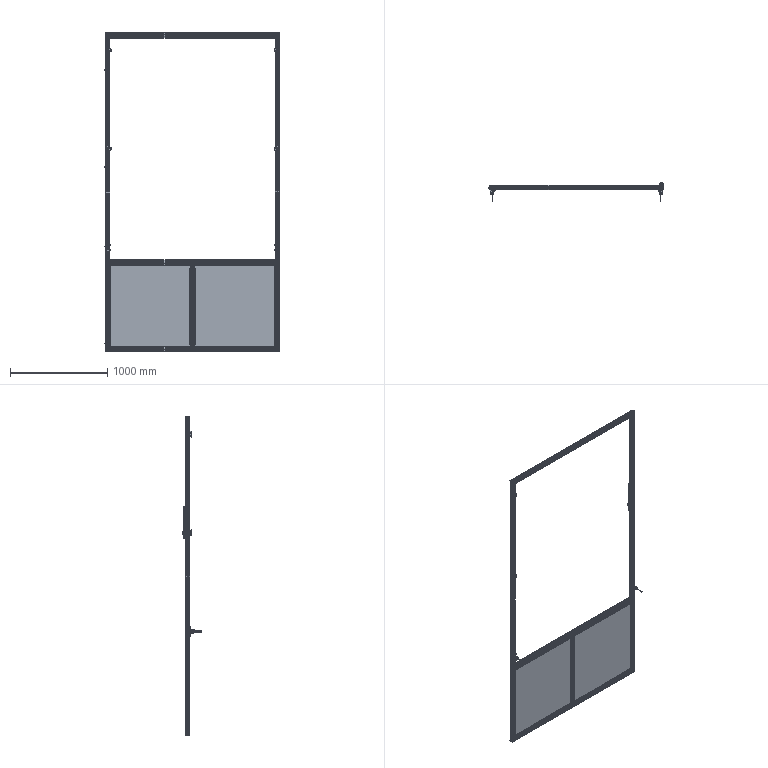Part | SolidWorks | features ReferencePattern 57, LocalLPattern 5, CompositeCurve 3 | 167 solids | 12893 faces | volume 16081270 mm3 | plane 8267 | cylinder 3118 | cone 856 | spline 592 | torus 48 | sphere 12 | commonest cylinder face diameters 6 x1712 2 x168 6.8 x151 5 x96 8 x94 4 x50